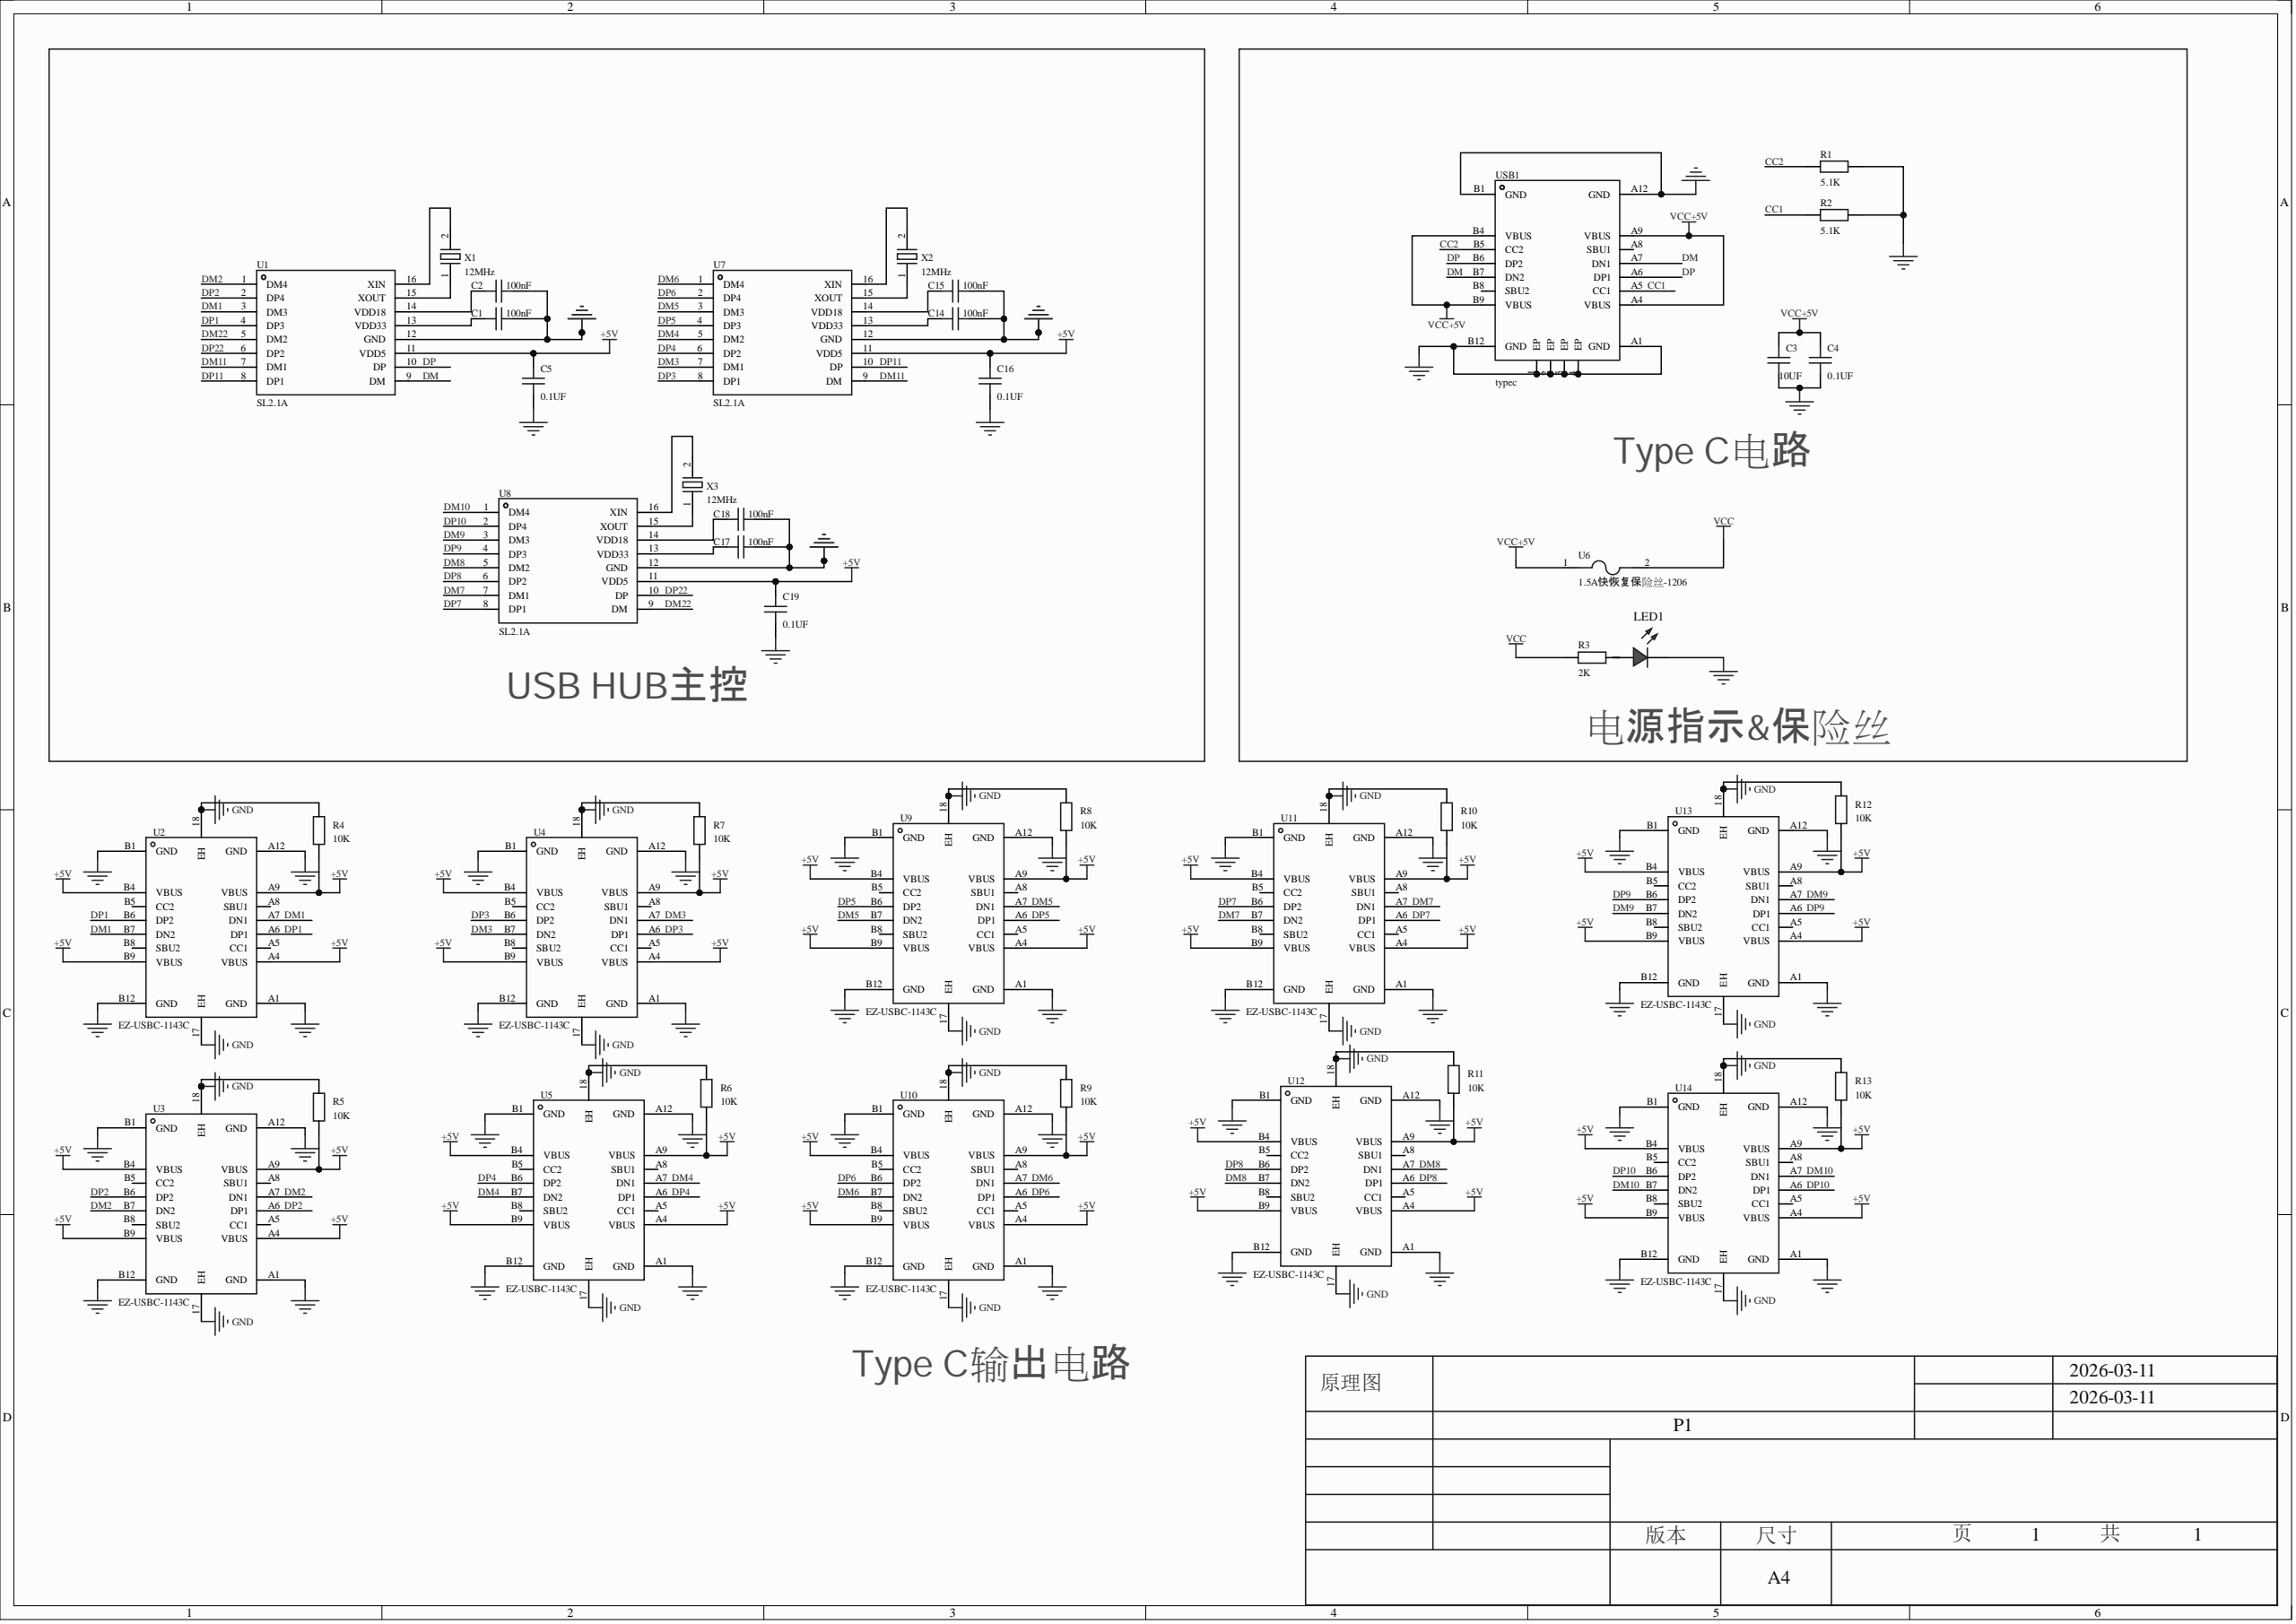Circuit board | Altium Designer | 43 parts | 45 nets
Bill of materials:
Comment,Description,Designator,Footprint,LibRef,Quantity
"100nF","","C1, C2, C14, C15, C17, C18","C0805","CAP_0805","6"
"10UF","","C3","C0805","CAP_0805","1"
"0.1UF","","C4, C5, C16, C19","C0805","CAP_0805","4"
"","","LED1","LED_0805","LED_0805-R","1"
"5.1K","","R1, R2","R0805","Res_0805","2"
"2K","","R3","R0805","Res_0805","1"
"10K","","R4, R5, R6, R7, R8, R9, R10, R11, R12, R13","R0603","Res_0603","10"
"SL2.1A","","U1, U7, U8","SOP-16_L10.0-W3.9-P1.27-LS6.0-BL","SL2.1A","3"
"EZ-USBC-1143C","","U2, U3, U4, U5, U9, U10, U11, U12, U13, U14","USB-SMD_EZ-USBC-1143C","EZ-USBC-1143C","10"
"1.5A快恢复保险丝-1206","","U6","F1206","1.5A快恢复保险丝-1206","1"
"typec","","USB1","USB-C-SMD_KH-TYPE-C-16P","typec","1"
"12MHz","","X1, X2, X3","CRYSTAL-SMD_L11.1-W4.8-LS12.3","9AT12000201060C3","3"
Netlist (Protel format):
[
C1
C0805
100nF



]
[
C2
C0805
100nF



]
[
C3
C0805
10UF



]
[
C4
C0805
0.1UF



]
[
C5
C0805
0.1UF



]
[
C14
C0805
100nF



]
[
C15
C0805
100nF



]
[
C16
C0805
0.1UF



]
[
C17
C0805
100nF



]
[
C18
C0805
100nF



]
[
C19
C0805
0.1UF



]
[
LED1
LED_0805




]
[
R1
R0805
5.1K



]
[
R2
R0805
5.1K



]
[
R3
R0805
2K



]
[
R4
R0603
10K



]
[
R5
R0603
10K



]
[
R6
R0603
10K



]
[
R7
R0603
10K



]
[
R8
R0603
10K



]
[
R9
R0603
10K



]
[
R10
R0603
10K



]
[
R11
R0603
10K



]
[
R12
R0603
10K



]
[
R13
R0603
10K



]
[
U1
SOP-16_L10.0-W3.9-P1.27-LS6.0-BL
SL2.1A



]
[
U2
USB-SMD_EZ-USBC-1143C
EZ-USBC-1143C



]
[
U3
USB-SMD_EZ-USBC-1143C
EZ-USBC-1143C



]
[
U4
USB-SMD_EZ-USBC-1143C
EZ-USBC-1143C



]
[
U5
USB-SMD_EZ-USBC-1143C
EZ-USBC-1143C



]
[
U6
F1206
1.5A快恢复保险丝-1206



]
[
U7
SOP-16_L10.0-W3.9-P1.27-LS6.0-BL
SL2.1A



]
[
U8
SOP-16_L10.0-W3.9-P1.27-LS6.0-BL
SL2.1A



]
[
U9
USB-SMD_EZ-USBC-1143C
EZ-USBC-1143C



]
[
U10
USB-SMD_EZ-USBC-1143C
EZ-USBC-1143C



]
[
U11
USB-SMD_EZ-USBC-1143C
EZ-USBC-1143C



]
[
U12
USB-SMD_EZ-USBC-1143C
EZ-USBC-1143C



]
[
U13
USB-SMD_EZ-USBC-1143C
EZ-USBC-1143C



]
[
U14
USB-SMD_EZ-USBC-1143C
EZ-USBC-1143C



]
[
USB1
USB-C-SMD_KH-TYPE-C-16P
typec



]
[
X1
CRYSTAL-SMD_L11.1-W4.8-LS12.3
12MHz



]
[
X2
CRYSTAL-SMD_L11.1-W4.8-LS12.3
12MHz



]
[
X3
CRYSTAL-SMD_L11.1-W4.8-LS12.3
12MHz



]
(
VCC+5V
C3-2
C4-2
U6-1
USB1-A4
USB1-A9
USB1-B4
USB1-B9
)
(
VCC
R3-2
U6-2
)
(
NetU8_16
U8-16
X3-2
)
(
NetU8_15
U8-15
X3-1
)
(
NetU7_16
U7-16
X2-2
)
(
NetU7_15
U7-15
X2-1
)
(
NetU1_16
U1-16
X1-2
)
(
NetU1_15
U1-15
X1-1
)
(
NetLED1_2
LED1-2
R3-1
)
(
NetC18_1
C18-1
U8-14
)
(
NetC17_1
C17-1
U8-13
)
(
NetC15_1
C15-1
U7-14
)
(
NetC14_1
C14-1
U7-13
)
(
NetC2_1
C2-1
U1-14
)
(
NetC1_1
C1-1
U1-13
)
(
GND
C1-2
C2-2
C3-1
C4-1
C5-1
C14-2
C15-2
C16-1
C17-2
C18-2
C19-1
LED1-1
R1-2
R2-2
R4-2
R5-2
R6-2
R7-2
R8-2
R9-2
R10-2
R11-2
R12-2
R13-2
U1-12
U2-17
U2-18
U2-A1
U2-A12
U2-B1
U2-B12
U3-17
U3-18
U3-A1
U3-A12
U3-B1
U3-B12
U4-17
U4-18
U4-A1
U4-A12
U4-B1
U4-B12
U5-17
U5-18
U5-A1
U5-A12
U5-B1
U5-B12
U7-12
U8-12
U9-17
U9-18
U9-A1
U9-A12
U9-B1
U9-B12
U10-17
U10-18
U10-A1
U10-A12
U10-B1
U10-B12
U11-17
U11-18
U11-A1
U11-A12
U11-B1
U11-B12
U12-17
U12-18
U12-A1
U12-A12
U12-B1
U12-B12
U13-17
U13-18
U13-A1
U13-A12
U13-B1
U13-B12
U14-17
U14-18
U14-A1
U14-A12
U14-B1
U14-B12
USB1-1
USB1-2
USB1-3
USB1-4
USB1-A1
USB1-A12
USB1-B1
USB1-B12
)
(
DP22
U1-6
U8-10
)
(
DP11
U1-8
U7-10
)
(
DP10
U8-2
U14-A6
U14-B6
)
(
DP9
U8-4
U13-A6
U13-B6
)
(
DP8
U8-6
U12-A6
U12-B6
)
(
DP7
U8-8
U11-A6
U11-B6
)
(
DP6
U7-2
U10-A6
U10-B6
)
(
DP5
U7-4
U9-A6
U9-B6
)
(
DP4
U5-A6
U5-B6
U7-6
)
(
DP3
U4-A6
U4-B6
U7-8
)
(
DP2
U1-2
U3-A6
U3-B6
)
(
DP1
U1-4
U2-A6
U2-B6
)
(
DP
U1-10
USB1-A6
USB1-B6
)
(
DM22
U1-5
U8-9
)
(
DM11
U1-7
U7-9
)
(
DM10
U8-1
U14-A7
U14-B7
)
(
DM9
U8-3
U13-A7
U13-B7
)
(
DM8
U8-5
U12-A7
U12-B7
)
(
DM7
U8-7
U11-A7
U11-B7
)
(
DM6
U7-1
U10-A7
U10-B7
)
(
DM5
U7-3
U9-A7
U9-B7
)
(
DM4
U5-A7
U5-B7
U7-5
)
(
DM3
U4-A7
U4-B7
U7-7
)
(
DM2
U1-1
U3-A7
U3-B7
)
(
DM1
U1-3
U2-A7
U2-B7
)
(
DM
U1-9
USB1-A7
USB1-B7
)
(
CC2
R1-1
USB1-B5
)
(
CC1
R2-1
USB1-A5
)
(
+5V
C5-2
C16-2
C19-2
R4-1
R5-1
R6-1
R7-1
R8-1
R9-1
R10-1
R11-1
R12-1
R13-1
U1-11
U2-A4
U2-A9
U2-B4
U2-B9
U3-A4
U3-A9
U3-B4
U3-B9
U4-A4
U4-A9
U4-B4
U4-B9
U5-A4
U5-A9
U5-B4
U5-B9
U7-11
U8-11
U9-A4
U9-A9
U9-B4
U9-B9
U10-A4
U10-A9
U10-B4
U10-B9
U11-A4
U11-A9
U11-B4
U11-B9
U12-A4
U12-A9
U12-B4
U12-B9
U13-A4
U13-A9
U13-B4
U13-B9
U14-A4
U14-A9
U14-B4
U14-B9
)